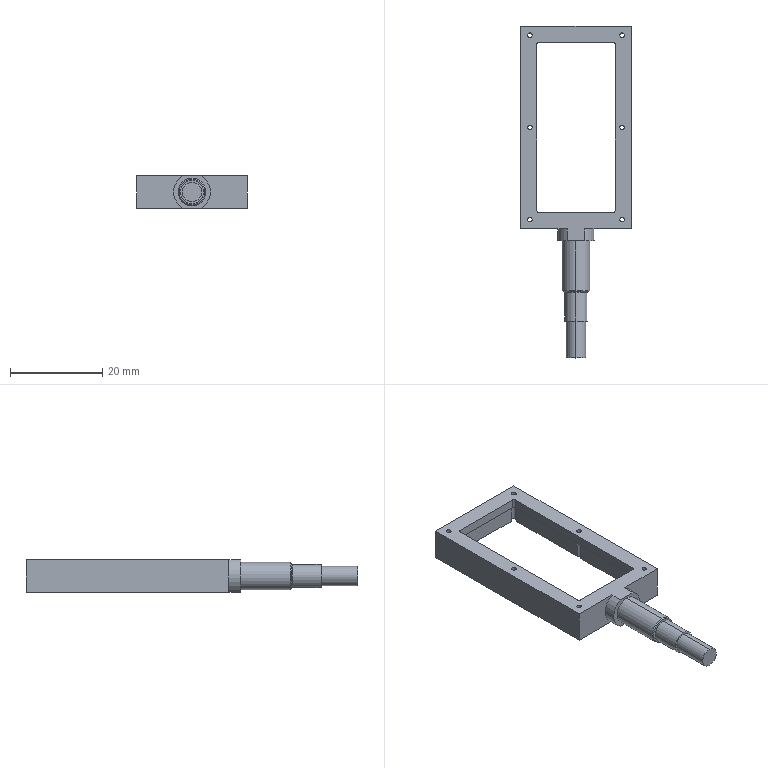NC program | NX | posted with a generic post | part box 24 x 72 x 7 mm
Lines 2081 to 3155 of 5160:
(CAVITY_MILL_COPY_COPY_COPY , TOOL : D1)
N4124 T01 M6
N4126 G54
N4128 G17 G0 G90 X-9.3 Y3.859 S9500 M3
N4130 G43 Z30. H1
N4132 Z-8.079
N4134 G94 G1 Z-9.079 F1000.
N4136 G3 X-9.5 Y3.259 R1.
N4138 G1 Y2.866 F800.
N4140 G2 X-9.634 Y2.366 R1.
N4142 X-9.134 Y2.5 R1.
N4144 G1 X-8.741
N4146 G3 X-8.141 Y2.7 R1.
N4148 G1 Z-8.079
N4150 G0 Z30.
N4152 X-9.3 Y3.859
N4154 Z-8.159
N4156 G1 Z-9.159 F1000.
N4158 G3 X-9.5 Y3.259 R1.
N4160 G1 Y2.866 F800.
N4162 G2 X-9.634 Y2.366 R1.
N4164 X-9.134 Y2.5 R1.
N4166 G1 X-8.741
N4168 G3 X-8.141 Y2.7 R1.
N4170 G1 Z-8.159
N4172 G0 Z30.
N4174 X-9.3 Y3.859
N4176 Z-8.238
N4178 G1 Z-9.238 F1000.
N4180 G3 X-9.5 Y3.259 R1.
N4182 G1 Y2.866 F800.
N4184 G2 X-9.634 Y2.366 R1.
N4186 X-9.134 Y2.5 R1.
N4188 G1 X-8.741
N4190 G3 X-8.141 Y2.7 R1.
N4192 G1 Z-8.238
N4194 G0 Z30.
N4196 X-9.3 Y3.859
N4198 Z-8.317
N4200 G1 Z-9.317 F1000.
N4202 G3 X-9.5 Y3.259 R1.
N4204 G1 Y2.866 F800.
N4206 G2 X-9.634 Y2.366 R1.
N4208 X-9.134 Y2.5 R1.
N4210 G1 X-8.741
N4212 G3 X-8.141 Y2.7 R1.
N4214 G1 Z-8.317
N4216 G0 Z30.
N4218 X-9.3 Y3.859
N4220 Z-8.397
N4222 G1 Z-9.397 F1000.
N4224 G3 X-9.5 Y3.259 R1.
N4226 G1 Y2.866 F800.
N4228 G2 X-9.634 Y2.366 R1.
N4230 X-9.134 Y2.5 R1.
N4232 G1 X-8.741
N4234 G3 X-8.141 Y2.7 R1.
N4236 G1 Z-8.397
N4238 G0 Z30.
N4240 X-9.3 Y3.859
N4242 Z-8.476
N4244 G1 Z-9.476 F1000.
N4246 G3 X-9.5 Y3.259 R1.
N4248 G1 Y2.866 F800.
N4250 G2 X-9.634 Y2.366 R1.
N4252 X-9.134 Y2.5 R1.
N4254 G1 X-8.741
N4256 G3 X-8.141 Y2.7 R1.
N4258 G1 Z-8.476
N4260 G0 Z30.
N4262 X-9.3 Y3.859
N4264 Z-8.556
N4266 G1 Z-9.556 F1000.
N4268 G3 X-9.5 Y3.259 R1.
N4270 G1 Y2.866 F800.
N4272 G2 X-9.634 Y2.366 R1.
N4274 X-9.134 Y2.5 R1.
N4276 G1 X-8.741
N4278 G3 X-8.141 Y2.7 R1.
N4280 G1 Z-8.556
N4282 G0 Z30.
N4284 X-9.3 Y3.859
N4286 Z-8.635
N4288 G1 Z-9.635 F1000.
N4290 G3 X-9.5 Y3.259 R1.
N4292 G1 Y2.866 F800.
N4294 G2 X-9.634 Y2.366 R1.
N4296 X-9.134 Y2.5 R1.
N4298 G1 X-8.741
N4300 G3 X-8.141 Y2.7 R1.
N4302 G1 Z-8.635
N4304 G0 Z30.
N4306 X-9.3 Y3.859
N4308 Z-8.714
N4310 G1 Z-9.714 F1000.
N4312 G3 X-9.5 Y3.259 R1.
N4314 G1 Y2.866 F800.
N4316 G2 X-9.634 Y2.366 R1.
N4318 X-9.134 Y2.5 R1.
N4320 G1 X-8.741
N4322 G3 X-8.141 Y2.7 R1.
N4324 G1 Z-8.714
N4326 G0 Z30.
N4328 X-9.3 Y3.859
N4330 Z-8.794
N4332 G1 Z-9.794 F1000.
N4334 G3 X-9.5 Y3.259 R1.
N4336 G1 Y2.866 F800.
N4338 G2 X-9.634 Y2.366 R1.
N4340 X-9.134 Y2.5 R1.
N4342 G1 X-8.741
N4344 G3 X-8.141 Y2.7 R1.
N4346 G1 Z-8.794
N4348 G0 Z30.
N4350 X-9.3 Y3.859
N4352 Z-8.873
N4354 G1 Z-9.873 F1000.
N4356 G3 X-9.5 Y3.259 R1.
N4358 G1 Y2.866 F800.
N4360 G2 X-9.634 Y2.366 R1.
N4362 X-9.134 Y2.5 R1.
N4364 G1 X-8.741
N4366 G3 X-8.141 Y2.7 R1.
N4368 G1 Z-8.873
N4370 G0 Z30.
N4372 X-9.3 Y3.859
N4374 Z-8.952
N4376 G1 Z-9.952 F1000.
N4378 G3 X-9.5 Y3.259 R1.
N4380 G1 Y2.866 F800.
N4382 G2 X-9.634 Y2.366 R1.
N4384 X-9.134 Y2.5 R1.
N4386 G1 X-8.741
N4388 G3 X-8.141 Y2.7 R1.
N4390 G1 Z-8.952
N4392 G0 X-9.3 Y3.859 Z-9.032
N4394 G1 Z-10.032 F1000.
N4396 G3 X-9.5 Y3.259 R1.
N4398 G1 Y2.866 F800.
N4400 G2 X-9.634 Y2.366 R1.
N4402 X-9.134 Y2.5 R1.
N4404 G1 X-8.741
N4406 G3 X-8.141 Y2.7 R1.
N4408 G1 Z-9.032
N4410 G0 X-9.3 Y3.859 Z-9.111
N4412 G1 Z-10.111 F1000.
N4414 G3 X-9.5 Y3.259 R1.
N4416 G1 Y2.866 F800.
N4418 G2 X-9.634 Y2.366 R1.
N4420 X-9.134 Y2.5 R1.
N4422 G1 X-8.741
N4424 G3 X-8.141 Y2.7 R1.
N4426 G1 Z-9.111
N4428 G0 X-9.3 Y3.859 Z-9.19
N4430 G1 Z-10.19 F1000.
N4432 G3 X-9.5 Y3.259 R1.
N4434 G1 Y2.866 F800.
N4436 G2 X-9.634 Y2.366 R1.
N4438 X-9.134 Y2.5 R1.
N4440 G1 X-8.741
N4442 G3 X-8.141 Y2.7 R1.
N4444 G1 Z-9.19
N4446 G0 X-9.3 Y3.859 Z-9.27
N4448 G1 Z-10.27 F1000.
N4450 G3 X-9.5 Y3.259 R1.
N4452 G1 Y2.866 F800.
N4454 G2 X-9.634 Y2.366 R1.
N4456 X-9.134 Y2.5 R1.
N4458 G1 X-8.741
N4460 G3 X-8.141 Y2.7 R1.
N4462 G1 Z-9.27
N4464 G0 X-9.3 Y3.859 Z-9.349
N4466 G1 Z-10.349 F1000.
N4468 G3 X-9.5 Y3.259 R1.
N4470 G1 Y2.866 F800.
N4472 G2 X-9.634 Y2.366 R1.
N4474 X-9.134 Y2.5 R1.
N4476 G1 X-8.741
N4478 G3 X-8.141 Y2.7 R1.
N4480 G1 Z-9.349
N4482 G0 X-9.3 Y3.859 Z-9.429
N4484 G1 Z-10.429 F1000.
N4486 G3 X-9.5 Y3.259 R1.
N4488 G1 Y2.866 F800.
N4490 G2 X-9.634 Y2.366 R1.
N4492 X-9.134 Y2.5 R1.
N4494 G1 X-8.741
N4496 G3 X-8.141 Y2.7 R1.
N4498 G1 Z-9.429
N4500 G0 X-9.3 Y3.859 Z-9.508
N4502 G1 Z-10.508 F1000.
N4504 G3 X-9.5 Y3.259 R1.
N4506 G1 Y2.866 F800.
N4508 G2 X-9.634 Y2.366 R1.
N4510 X-9.134 Y2.5 R1.
N4512 G1 X-8.741
N4514 G3 X-8.141 Y2.7 R1.
N4516 G1 Z-9.508
N4518 G0 X-9.3 Y3.859 Z-9.587
N4520 G1 Z-10.587 F1000.
N4522 G3 X-9.5 Y3.259 R1.
N4524 G1 Y2.866 F800.
N4526 G2 X-9.634 Y2.366 R1.
N4528 X-9.134 Y2.5 R1.
N4530 G1 X-8.741
N4532 G3 X-8.141 Y2.7 R1.
N4534 G1 Z-9.587
N4536 G0 X-9.3 Y3.859 Z-9.667
N4538 G1 Z-10.667 F1000.
N4540 G3 X-9.5 Y3.259 R1.
N4542 G1 Y2.866 F800.
N4544 G2 X-9.634 Y2.366 R1.
N4546 X-9.134 Y2.5 R1.
N4548 G1 X-8.741
N4550 G3 X-8.141 Y2.7 R1.
N4552 G1 Z-9.667
N4554 G0 X-9.3 Y3.859 Z-9.746
N4556 G1 Z-10.746 F1000.
N4558 G3 X-9.5 Y3.259 R1.
N4560 G1 Y2.866 F800.
N4562 G2 X-9.634 Y2.366 R1.
N4564 X-9.134 Y2.5 R1.
N4566 G1 X-8.741
N4568 G3 X-8.141 Y2.7 R1.
N4570 G1 Z-9.746
N4572 G0 X-9.3 Y3.859 Z-9.825
N4574 G1 Z-10.825 F1000.
N4576 G3 X-9.5 Y3.259 R1.
N4578 G1 Y2.866 F800.
N4580 G2 X-9.634 Y2.366 R1.
N4582 X-9.134 Y2.5 R1.
N4584 G1 X-8.741
N4586 G3 X-8.141 Y2.7 R1.
N4588 G1 Z-9.825
N4590 G0 X-9.3 Y3.859 Z-9.905
N4592 G1 Z-10.905 F1000.
N4594 G3 X-9.5 Y3.259 R1.
N4596 G1 Y2.866 F800.
N4598 G2 X-9.634 Y2.366 R1.
N4600 X-9.134 Y2.5 R1.
N4602 G1 X-8.741
N4604 G3 X-8.141 Y2.7 R1.
N4606 G1 Z-9.905
N4608 G0 X-9.3 Y3.859 Z-9.984
N4610 G1 Z-10.984 F1000.
N4612 G3 X-9.5 Y3.259 R1.
N4614 G1 Y2.866 F800.
N4616 G2 X-9.634 Y2.366 R1.
N4618 X-9.134 Y2.5 R1.
N4620 G1 X-8.741
N4622 G3 X-8.141 Y2.7 R1.
N4624 G1 Z-9.984
N4626 G0 X-9.3 Y3.859 Z-10.063
N4628 G1 Z-11.063 F1000.
N4630 G3 X-9.5 Y3.259 R1.
N4632 G1 Y2.866 F800.
N4634 G2 X-9.634 Y2.366 R1.
N4636 X-9.134 Y2.5 R1.
N4638 G1 X-8.741
N4640 G3 X-8.141 Y2.7 R1.
N4642 G1 Z-10.063
N4644 G0 X-9.3 Y3.859 Z-10.143
N4646 G1 Z-11.143 F1000.
N4648 G3 X-9.5 Y3.259 R1.
N4650 G1 Y2.866 F800.
N4652 G2 X-9.634 Y2.366 R1.
N4654 X-9.134 Y2.5 R1.
N4656 G1 X-8.741
N4658 G3 X-8.141 Y2.7 R1.
N4660 G1 Z-10.143
N4662 G0 X-9.3 Y3.859 Z-10.222
N4664 G1 Z-11.222 F1000.
N4666 G3 X-9.5 Y3.259 R1.
N4668 G1 Y2.866 F800.
N4670 G2 X-9.634 Y2.366 R1.
N4672 X-9.134 Y2.5 R1.
N4674 G1 X-8.741
N4676 G3 X-8.141 Y2.7 R1.
N4678 G1 Z-10.222
N4680 G0 X-9.3 Y3.859 Z-10.302
N4682 G1 Z-11.302 F1000.
N4684 G3 X-9.5 Y3.259 R1.
N4686 G1 Y2.866 F800.
N4688 G2 X-9.634 Y2.366 R1.
N4690 X-9.134 Y2.5 R1.
N4692 G1 X-8.741
N4694 G3 X-8.141 Y2.7 R1.
N4696 G1 Z-10.302
N4698 G0 X-9.3 Y3.859 Z-10.381
N4700 G1 Z-11.381 F1000.
N4702 G3 X-9.5 Y3.259 R1.
N4704 G1 Y2.866 F800.
N4706 G2 X-9.634 Y2.366 R1.
N4708 X-9.134 Y2.5 R1.
N4710 G1 X-8.741
N4712 G3 X-8.141 Y2.7 R1.
N4714 G1 Z-10.381
N4716 G0 X-9.3 Y3.859 Z-10.46
N4718 G1 Z-11.46 F1000.
N4720 G3 X-9.5 Y3.259 R1.
N4722 G1 Y2.866 F800.
N4724 G2 X-9.634 Y2.366 R1.
N4726 X-9.134 Y2.5 R1.
N4728 G1 X-8.741
N4730 G3 X-8.141 Y2.7 R1.
N4732 G1 Z-10.46
N4734 G0 X-9.3 Y3.859 Z-10.54
N4736 G1 Z-11.54 F1000.
N4738 G3 X-9.5 Y3.259 R1.
N4740 G1 Y2.866 F800.
N4742 G2 X-9.634 Y2.366 R1.
N4744 X-9.134 Y2.5 R1.
N4746 G1 X-8.741
N4748 G3 X-8.141 Y2.7 R1.
N4750 G1 Z-10.54
N4752 G0 X-9.3 Y3.859 Z-10.619
N4754 G1 Z-11.619 F1000.
N4756 G3 X-9.5 Y3.259 R1.
N4758 G1 Y2.866 F800.
N4760 G2 X-9.634 Y2.366 R1.
N4762 X-9.134 Y2.5 R1.
N4764 G1 X-8.741
N4766 G3 X-8.141 Y2.7 R1.
N4768 G1 Z-10.619
N4770 G0 X-9.3 Y3.859 Z-10.698
N4772 G1 Z-11.698 F1000.
N4774 G3 X-9.5 Y3.259 R1.
N4776 G1 Y2.866 F800.
N4778 G2 X-9.634 Y2.366 R1.
N4780 X-9.134 Y2.5 R1.
N4782 G1 X-8.741
N4784 G3 X-8.141 Y2.7 R1.
N4786 G1 Z-10.698
N4788 G0 X-9.3 Y3.859 Z-10.778
N4790 G1 Z-11.778 F1000.
N4792 G3 X-9.5 Y3.259 R1.
N4794 G1 Y2.866 F800.
N4796 G2 X-9.634 Y2.366 R1.
N4798 X-9.134 Y2.5 R1.
N4800 G1 X-8.741
N4802 G3 X-8.141 Y2.7 R1.
N4804 G1 Z-10.778
N4806 G0 X-9.3 Y3.859 Z-10.857
N4808 G1 Z-11.857 F1000.
N4810 G3 X-9.5 Y3.259 R1.
N4812 G1 Y2.866 F800.
N4814 G2 X-9.634 Y2.366 R1.
N4816 X-9.134 Y2.5 R1.
N4818 G1 X-8.741
N4820 G3 X-8.141 Y2.7 R1.
N4822 G1 Z-10.857
N4824 G0 X-9.3 Y3.859 Z-10.937
N4826 G1 Z-11.937 F1000.
N4828 G3 X-9.5 Y3.259 R1.
N4830 G1 Y2.866 F800.
N4832 G2 X-9.634 Y2.366 R1.
N4834 X-9.134 Y2.5 R1.
N4836 G1 X-8.741
N4838 G3 X-8.141 Y2.7 R1.
N4840 G1 Z-10.937
N4842 G0 X-9.3 Y3.859 Z-11.016
N4844 G1 Z-12.016 F1000.
N4846 G3 X-9.5 Y3.259 R1.
N4848 G1 Y2.866 F800.
N4850 G2 X-9.634 Y2.366 R1.
N4852 X-9.134 Y2.5 R1.
N4854 G1 X-8.741
N4856 G3 X-8.141 Y2.7 R1.
N4858 G1 Z-11.016
N4860 G0 X-9.3 Y3.859 Z-11.095
N4862 G1 Z-12.095 F1000.
N4864 G3 X-9.5 Y3.259 R1.
N4866 G1 Y2.866 F800.
N4868 G2 X-9.634 Y2.366 R1.
N4870 X-9.134 Y2.5 R1.
N4872 G1 X-8.741
N4874 G3 X-8.141 Y2.7 R1.
N4876 G1 Z-11.095
N4878 G0 X-9.3 Y3.859 Z-11.175
N4880 G1 Z-12.175 F1000.
N4882 G3 X-9.5 Y3.259 R1.
N4884 G1 Y2.866 F800.
N4886 G2 X-9.634 Y2.366 R1.
N4888 X-9.134 Y2.5 R1.
N4890 G1 X-8.741
N4892 G3 X-8.141 Y2.7 R1.
N4894 G1 Z-11.175
N4896 G0 X-9.3 Y3.859 Z-11.254
N4898 G1 Z-12.254 F1000.
N4900 G3 X-9.5 Y3.259 R1.
N4902 G1 Y2.866 F800.
N4904 G2 X-9.634 Y2.366 R1.
N4906 X-9.134 Y2.5 R1.
N4908 G1 X-8.741
N4910 G3 X-8.141 Y2.7 R1.
N4912 G1 Z-11.254
N4914 G0 X-9.3 Y3.859 Z-11.333
N4916 G1 Z-12.333 F1000.
N4918 G3 X-9.5 Y3.259 R1.
N4920 G1 Y2.866 F800.
N4922 G2 X-9.634 Y2.366 R1.
N4924 X-9.134 Y2.5 R1.
N4926 G1 X-8.741
N4928 G3 X-8.141 Y2.7 R1.
N4930 G1 Z-11.333
N4932 G0 X-9.3 Y3.859 Z-11.413
N4934 G1 Z-12.413 F1000.
N4936 G3 X-9.5 Y3.259 R1.
N4938 G1 Y2.866 F800.
N4940 G2 X-9.634 Y2.366 R1.
N4942 X-9.134 Y2.5 R1.
N4944 G1 X-8.741
N4946 G3 X-8.141 Y2.7 R1.
N4948 G1 Z-11.413
N4950 G0 X-9.3 Y3.859 Z-11.492
N4952 G1 Z-12.492 F1000.
N4954 G3 X-9.5 Y3.259 R1.
N4956 G1 Y2.866 F800.
N4958 G2 X-9.634 Y2.366 R1.
N4960 X-9.134 Y2.5 R1.
N4962 G1 X-8.741
N4964 G3 X-8.141 Y2.7 R1.
N4966 G1 Z-11.492
N4968 G0 X-9.3 Y3.859 Z-11.571
N4970 G1 Z-12.571 F1000.
N4972 G3 X-9.5 Y3.259 R1.
N4974 G1 Y2.866 F800.
N4976 G2 X-9.634 Y2.366 R1.
N4978 X-9.134 Y2.5 R1.
N4980 G1 X-8.741
N4982 G3 X-8.141 Y2.7 R1.
N4984 G1 Z-11.571
N4986 G0 X-9.3 Y3.859 Z-11.651
N4988 G1 Z-12.651 F1000.
N4990 G3 X-9.5 Y3.259 R1.
N4992 G1 Y2.866 F800.
N4994 G2 X-9.634 Y2.366 R1.
N4996 X-9.134 Y2.5 R1.
N4998 G1 X-8.741
N5000 G3 X-8.141 Y2.7 R1.
N5002 G1 Z-11.651
N5004 G0 X-9.3 Y3.859 Z-11.73
N5006 G1 Z-12.73 F1000.
N5008 G3 X-9.5 Y3.259 R1.
N5010 G1 Y2.866 F800.
N5012 G2 X-9.634 Y2.366 R1.
N5014 X-9.134 Y2.5 R1.
N5016 G1 X-8.741
N5018 G3 X-8.141 Y2.7 R1.
N5020 G1 Z-11.73
N5022 G0 X-9.3 Y3.859 Z-11.81
N5024 G1 Z-12.81 F1000.
N5026 G3 X-9.5 Y3.259 R1.
N5028 G1 Y2.866 F800.
N5030 G2 X-9.634 Y2.366 R1.
N5032 X-9.134 Y2.5 R1.
N5034 G1 X-8.741
N5036 G3 X-8.141 Y2.7 R1.
N5038 G1 Z-11.81
N5040 G0 X-9.3 Y3.859 Z-11.889
N5042 G1 Z-12.889 F1000.
N5044 G3 X-9.5 Y3.259 R1.
N5046 G1 Y2.866 F800.
N5048 G2 X-9.634 Y2.366 R1.
N5050 X-9.134 Y2.5 R1.
N5052 G1 X-8.741
N5054 G3 X-8.141 Y2.7 R1.
N5056 G1 Z-11.889
N5058 G0 X-9.3 Y3.859 Z-11.968
N5060 G1 Z-12.968 F1000.
N5062 G3 X-9.5 Y3.259 R1.
N5064 G1 Y2.866 F800.
N5066 G2 X-9.634 Y2.366 R1.
N5068 X-9.134 Y2.5 R1.
N5070 G1 X-8.741
N5072 G3 X-8.141 Y2.7 R1.
N5074 G1 Z-11.968
N5076 G0 X-9.3 Y3.859 Z-12.048
N5078 G1 Z-13.048 F1000.
N5080 G3 X-9.5 Y3.259 R1.
N5082 G1 Y2.866 F800.
N5084 G2 X-9.634 Y2.366 R1.
N5086 X-9.134 Y2.5 R1.
N5088 G1 X-8.741
N5090 G3 X-8.141 Y2.7 R1.
N5092 G1 Z-12.048
N5094 G0 X-9.3 Y3.859 Z-12.127
N5096 G1 Z-13.127 F1000.
N5098 G3 X-9.5 Y3.259 R1.
N5100 G1 Y2.866 F800.
N5102 G2 X-9.634 Y2.366 R1.
N5104 X-9.134 Y2.5 R1.
N5106 G1 X-8.741
N5108 G3 X-8.141 Y2.7 R1.
N5110 G1 Z-12.127
N5112 G0 X-9.3 Y3.859 Z-12.206
N5114 G1 Z-13.206 F1000.
N5116 G3 X-9.5 Y3.259 R1.
N5118 G1 Y2.866 F800.
N5120 G2 X-9.634 Y2.366 R1.
N5122 X-9.134 Y2.5 R1.
N5124 G1 X-8.741
N5126 G3 X-8.141 Y2.7 R1.
N5128 G1 Z-12.206
N5130 G0 X-9.3 Y3.859 Z-12.286
N5132 G1 Z-13.286 F1000.
N5134 G3 X-9.5 Y3.259 R1.
N5136 G1 Y2.866 F800.
N5138 G2 X-9.634 Y2.366 R1.
N5140 X-9.134 Y2.5 R1.
N5142 G1 X-8.741
N5144 G3 X-8.141 Y2.7 R1.
N5146 G1 Z-12.286
N5148 G0 X-9.3 Y3.859 Z-12.365
N5150 G1 Z-13.365 F1000.
N5152 G3 X-9.5 Y3.259 R1.
N5154 G1 Y2.866 F800.
N5156 G2 X-9.634 Y2.366 R1.
N5158 X-9.134 Y2.5 R1.
N5160 G1 X-8.741
N5162 G3 X-8.141 Y2.7 R1.
N5164 G1 Z-12.365
N5166 G0 X-9.3 Y3.859 Z-12.444
N5168 G1 Z-13.444 F1000.
N5170 G3 X-9.5 Y3.259 R1.
N5172 G1 Y2.866 F800.
N5174 G2 X-9.634 Y2.366 R1.
N5176 X-9.134 Y2.5 R1.
N5178 G1 X-8.741
N5180 G3 X-8.141 Y2.7 R1.
N5182 G1 Z-12.444
N5184 G0 X-9.3 Y3.859 Z-12.524
N5186 G1 Z-13.524 F1000.
N5188 G3 X-9.5 Y3.259 R1.
N5190 G1 Y2.866 F800.
N5192 G2 X-9.634 Y2.366 R1.
N5194 X-9.134 Y2.5 R1.
N5196 G1 X-8.741
N5198 G3 X-8.141 Y2.7 R1.
N5200 G1 Z-12.524
N5202 G0 X-9.3 Y3.859 Z-12.603
N5204 G1 Z-13.603 F1000.
N5206 G3 X-9.5 Y3.259 R1.
N5208 G1 Y2.866 F800.
N5210 G2 X-9.634 Y2.366 R1.
N5212 X-9.134 Y2.5 R1.
N5214 G1 X-8.741
N5216 G3 X-8.141 Y2.7 R1.
N5218 G1 Z-12.603
N5220 G0 X-9.3 Y3.859 Z-12.683
N5222 G1 Z-13.683 F1000.
N5224 G3 X-9.5 Y3.259 R1.
N5226 G1 Y2.866 F800.
N5228 G2 X-9.634 Y2.366 R1.
N5230 X-9.134 Y2.5 R1.
N5232 G1 X-8.741
N5234 G3 X-8.141 Y2.7 R1.
N5236 G1 Z-12.683
N5238 G0 X-9.3 Y3.859 Z-12.762
N5240 G1 Z-13.762 F1000.
N5242 G3 X-9.5 Y3.259 R1.
N5244 G1 Y2.866 F800.
N5246 G2 X-9.634 Y2.366 R1.
N5248 X-9.134 Y2.5 R1.
N5250 G1 X-8.741
N5252 G3 X-8.141 Y2.7 R1.
N5254 G1 Z-12.762
N5256 G0 X-9.3 Y3.859 Z-12.841
N5258 G1 Z-13.841 F1000.
N5260 G3 X-9.5 Y3.259 R1.
N5262 G1 Y2.866 F800.
N5264 G2 X-9.634 Y2.366 R1.
N5266 X-9.134 Y2.5 R1.
N5268 G1 X-8.741
N5270 G3 X-8.141 Y2.7 R1.
N5272 G1 Z-12.841
N5274 G0 X-9.3 Y3.859 Z-12.921
N5276 G1 Z-13.921 F1000.
N5278 G3 X-9.5 Y3.259 R1.
N5280 G1 Y2.866 F800.
N5282 G2 X-9.634 Y2.366 R1.
N5284 X-9.134 Y2.5 R1.
N5286 G1 X-8.741
N5288 G3 X-8.141 Y2.7 R1.
N5290 G1 Z-12.921
N5292 G0 X-9.3 Y3.859 Z-13.
N5294 G1 Z-14. F1000.
N5296 G3 X-9.5 Y3.259 R1.
N5298 G1 Y2.866 F800.
N5300 G2 X-9.634 Y2.366 R1.
N5302 X-9.134 Y2.5 R1.
N5304 G1 X-8.741
N5306 G3 X-8.141 Y2.7 R1.
N5308 G1 Z-13.
N5310 G0 Z30.
N5312 X-7.8 Y5.348
N5314 Z-13.08
N5316 G1 Z-14.08 F1000.
N5318 G3 X-8. Y4.748 R1.
N5320 G1 Y4. F800.
N5322 X-7.252
N5324 G3 X-6.652 Y4.2 R1.
N5326 G1 Z-13.08
N5328 G0 X-7.8 Y5.348 Z-13.16
N5330 G1 Z-14.16 F1000.
N5332 G3 X-8. Y4.748 R1.
N5334 G1 Y4. F800.
N5336 X-7.252
N5338 G3 X-6.652 Y4.2 R1.
N5340 G1 Z-13.16
N5342 G0 X-7.8 Y5.348 Z-13.24
N5344 G1 Z-14.24 F1000.
N5346 G3 X-8. Y4.748 R1.
N5348 G1 Y4. F800.
N5350 X-7.252
N5352 G3 X-6.652 Y4.2 R1.
N5354 G1 Z-13.24
N5356 G0 X-7.8 Y5.348 Z-13.32
N5358 G1 Z-14.32 F1000.
N5360 G3 X-8. Y4.748 R1.
N5362 G1 Y4. F800.
N5364 X-7.252
N5366 G3 X-6.652 Y4.2 R1.
N5368 G1 Z-13.32
N5370 G0 X-7.8 Y5.348 Z-13.4
N5372 G1 Z-14.4 F1000.
N5374 G3 X-8. Y4.748 R1.
N5376 G1 Y4. F800.
N5378 X-7.252
N5380 G3 X-6.652 Y4.2 R1.
N5382 G1 Z-13.4
N5384 G0 X-7.8 Y5.348 Z-13.48
N5386 G1 Z-14.48 F1000.
N5388 G3 X-8. Y4.748 R1.
N5390 G1 Y4. F800.
N5392 X-7.252
N5394 G3 X-6.652 Y4.2 R1.
N5396 G1 Z-13.48
N5398 G0 X-7.8 Y5.348 Z-13.56
N5400 G1 Z-14.56 F1000.
N5402 G3 X-8. Y4.748 R1.
N5404 G1 Y4. F800.
N5406 X-7.252
N5408 G3 X-6.652 Y4.2 R1.
N5410 G1 Z-13.56
N5412 G0 X-7.8 Y5.348 Z-13.64
N5414 G1 Z-14.64 F1000.
N5416 G3 X-8. Y4.748 R1.
N5418 G1 Y4. F800.
N5420 X-7.252
N5422 G3 X-6.652 Y4.2 R1.
N5424 G1 Z-13.64
N5426 G0 X-7.8 Y5.348 Z-13.72
N5428 G1 Z-14.72 F1000.
N5430 G3 X-8. Y4.748 R1.
N5432 G1 Y4. F800.
N5434 X-7.252
N5436 G3 X-6.652 Y4.2 R1.
N5438 G1 Z-13.72
N5440 G0 X-7.8 Y5.348 Z-13.8
N5442 G1 Z-14.8 F1000.
N5444 G3 X-8. Y4.748 R1.
N5446 G1 Y4. F800.
N5448 X-7.252
N5450 G3 X-6.652 Y4.2 R1.
N5452 G1 Z-13.8
N5454 G0 X-7.8 Y5.348 Z-13.88
N5456 G1 Z-14.88 F1000.
N5458 G3 X-8. Y4.748 R1.
N5460 G1 Y4. F800.
N5462 X-7.252
N5464 G3 X-6.652 Y4.2 R1.
N5466 G1 Z-13.88
N5468 G0 X-7.8 Y5.348 Z-13.96
N5470 G1 Z-14.96 F1000.
N5472 G3 X-8. Y4.748 R1.
N5474 G1 Y4. F800.
N5476 X-7.252
N5478 G3 X-6.652 Y4.2 R1.
N5480 G1 Z-13.96
N5482 G0 X-7.8 Y5.348 Z-14.04
N5484 G1 Z-15.04 F1000.
N5486 G3 X-8. Y4.748 R1.
N5488 G1 Y4. F800.
N5490 X-7.252
N5492 G3 X-6.652 Y4.2 R1.
N5494 G1 Z-14.04
N5496 G0 X-7.8 Y5.348 Z-14.12
N5498 G1 Z-15.12 F1000.
N5500 G3 X-8. Y4.748 R1.
N5502 G1 Y4. F800.
N5504 X-7.252
N5506 G3 X-6.652 Y4.2 R1.
N5508 G1 Z-14.12
N5510 G0 X-7.8 Y5.348 Z-14.2
N5512 G1 Z-15.2 F1000.
N5514 G3 X-8. Y4.748 R1.
N5516 G1 Y4. F800.
N5518 X-7.252
N5520 G3 X-6.652 Y4.2 R1.
N5522 G1 Z-14.2
N5524 G0 X-7.8 Y5.348 Z-14.28
N5526 G1 Z-15.28 F1000.
N5528 G3 X-8. Y4.748 R1.
N5530 G1 Y4. F800.
N5532 X-7.252
N5534 G3 X-6.652 Y4.2 R1.
N5536 G1 Z-14.28
N5538 G0 X-7.8 Y5.348 Z-14.36
N5540 G1 Z-15.36 F1000.
N5542 G3 X-8. Y4.748 R1.
N5544 G1 Y4. F800.
N5546 X-7.252
N5548 G3 X-6.652 Y4.2 R1.
N5550 G1 Z-14.36
N5552 G0 X-7.8 Y5.348 Z-14.44
N5554 G1 Z-15.44 F1000.
N5556 G3 X-8. Y4.748 R1.
N5558 G1 Y4. F800.
N5560 X-7.252
N5562 G3 X-6.652 Y4.2 R1.
N5564 G1 Z-14.44
N5566 G0 X-7.8 Y5.348 Z-14.52
N5568 G1 Z-15.52 F1000.
N5570 G3 X-8. Y4.748 R1.
N5572 G1 Y4. F800.
N5574 X-7.252
N5576 G3 X-6.652 Y4.2 R1.
N5578 G1 Z-14.52
N5580 G0 X-7.8 Y5.348 Z-14.6
N5582 G1 Z-15.6 F1000.
N5584 G3 X-8. Y4.748 R1.
N5586 G1 Y4. F800.
N5588 X-7.252
N5590 G3 X-6.652 Y4.2 R1.
N5592 G1 Z-14.6
N5594 G0 X-7.8 Y5.348 Z-14.68
N5596 G1 Z-15.68 F1000.
N5598 G3 X-8. Y4.748 R1.
N5600 G1 Y4. F800.
N5602 X-7.252
N5604 G3 X-6.652 Y4.2 R1.
N5606 G1 Z-14.68
N5608 G0 X-7.8 Y5.348 Z-14.76
N5610 G1 Z-15.76 F1000.
N5612 G3 X-8. Y4.748 R1.
N5614 G1 Y4. F800.
N5616 X-7.252
N5618 G3 X-6.652 Y4.2 R1.
N5620 G1 Z-14.76
N5622 G0 X-7.8 Y5.348 Z-14.84
N5624 G1 Z-15.84 F1000.
N5626 G3 X-8. Y4.748 R1.
N5628 G1 Y4. F800.
N5630 X-7.252
N5632 G3 X-6.652 Y4.2 R1.
N5634 G1 Z-14.84
N5636 G0 X-7.8 Y5.348 Z-14.92
N5638 G1 Z-15.92 F1000.
N5640 G3 X-8. Y4.748 R1.
N5642 G1 Y4. F800.
N5644 X-7.252
N5646 G3 X-6.652 Y4.2 R1.
N5648 G1 Z-14.92
N5650 G0 X-7.8 Y5.348 Z-15.
N5652 G1 Z-16. F1000.
N5654 G3 X-8. Y4.748 R1.
N5656 G1 Y4. F800.
N5658 X-7.252
N5660 G3 X-6.652 Y4.2 R1.
N5662 G1 Z-15.
N5664 G0 Z30.
N5666 X6.652
N5668 Z-13.08
N5670 G1 Z-14.08 F1000.
N5672 G3 X7.252 Y4. R1.
N5674 G1 X8. F800.
N5676 Y4.748
N5678 G3 X7.8 Y5.348 R1.
N5680 G1 Z-13.08
N5682 G0 X6.652 Y4.2 Z-13.16
N5684 G1 Z-14.16 F1000.
N5686 G3 X7.252 Y4. R1.
N5688 G1 X8. F800.
N5690 Y4.748
N5692 G3 X7.8 Y5.348 R1.
N5694 G1 Z-13.16
N5696 G0 X6.652 Y4.2 Z-13.24
N5698 G1 Z-14.24 F1000.
N5700 G3 X7.252 Y4. R1.
N5702 G1 X8. F800.
N5704 Y4.748
N5706 G3 X7.8 Y5.348 R1.
N5708 G1 Z-13.24
N5710 G0 X6.652 Y4.2 Z-13.32
N5712 G1 Z-14.32 F1000.
N5714 G3 X7.252 Y4. R1.
N5716 G1 X8. F800.
N5718 Y4.748
N5720 G3 X7.8 Y5.348 R1.
N5722 G1 Z-13.32
N5724 G0 X6.652 Y4.2 Z-13.4
N5726 G1 Z-14.4 F1000.
N5728 G3 X7.252 Y4. R1.
N5730 G1 X8. F800.
N5732 Y4.748
N5734 G3 X7.8 Y5.348 R1.
N5736 G1 Z-13.4
N5738 G0 X6.652 Y4.2 Z-13.48
N5740 G1 Z-14.48 F1000.
N5742 G3 X7.252 Y4. R1.
N5744 G1 X8. F800.
N5746 Y4.748
N5748 G3 X7.8 Y5.348 R1.
N5750 G1 Z-13.48
N5752 G0 X6.652 Y4.2 Z-13.56
N5754 G1 Z-14.56 F1000.
N5756 G3 X7.252 Y4. R1.
N5758 G1 X8. F800.
N5760 Y4.748
N5762 G3 X7.8 Y5.348 R1.
N5764 G1 Z-13.56
N5766 G0 X6.652 Y4.2 Z-13.64
N5768 G1 Z-14.64 F1000.
N5770 G3 X7.252 Y4. R1.
N5772 G1 X8. F800.
N5774 Y4.748
N5776 G3 X7.8 Y5.348 R1.
N5778 G1 Z-13.64
N5780 G0 X6.652 Y4.2 Z-13.72
N5782 G1 Z-14.72 F1000.
N5784 G3 X7.252 Y4. R1.
N5786 G1 X8. F800.
N5788 Y4.748
N5790 G3 X7.8 Y5.348 R1.
N5792 G1 Z-13.72
N5794 G0 X6.652 Y4.2 Z-13.8
N5796 G1 Z-14.8 F1000.
N5798 G3 X7.252 Y4. R1.
N5800 G1 X8. F800.
N5802 Y4.748
N5804 G3 X7.8 Y5.348 R1.
N5806 G1 Z-13.8
N5808 G0 X6.652 Y4.2 Z-13.88
N5810 G1 Z-14.88 F1000.
N5812 G3 X7.252 Y4. R1.
N5814 G1 X8. F800.
N5816 Y4.748
N5818 G3 X7.8 Y5.348 R1.
N5820 G1 Z-13.88
N5822 G0 X6.652 Y4.2 Z-13.96
N5824 G1 Z-14.96 F1000.
N5826 G3 X7.252 Y4. R1.
N5828 G1 X8. F800.
N5830 Y4.748
N5832 G3 X7.8 Y5.348 R1.
N5834 G1 Z-13.96
N5836 G0 X6.652 Y4.2 Z-14.04
N5838 G1 Z-15.04 F1000.
N5840 G3 X7.252 Y4. R1.
N5842 G1 X8. F800.
N5844 Y4.748
N5846 G3 X7.8 Y5.348 R1.
N5848 G1 Z-14.04
N5850 G0 X6.652 Y4.2 Z-14.12
N5852 G1 Z-15.12 F1000.
N5854 G3 X7.252 Y4. R1.
N5856 G1 X8. F800.
N5858 Y4.748
N5860 G3 X7.8 Y5.348 R1.
N5862 G1 Z-14.12
N5864 G0 X6.652 Y4.2 Z-14.2
N5866 G1 Z-15.2 F1000.
N5868 G3 X7.252 Y4. R1.
N5870 G1 X8. F800.
N5872 Y4.748
N5874 G3 X7.8 Y5.348 R1.
N5876 G1 Z-14.2
N5878 G0 X6.652 Y4.2 Z-14.28
N5880 G1 Z-15.28 F1000.
N5882 G3 X7.252 Y4. R1.
N5884 G1 X8. F800.
N5886 Y4.748
N5888 G3 X7.8 Y5.348 R1.
N5890 G1 Z-14.28
N5892 G0 X6.652 Y4.2 Z-14.36
N5894 G1 Z-15.36 F1000.
N5896 G3 X7.252 Y4. R1.
N5898 G1 X8. F800.
N5900 Y4.748
N5902 G3 X7.8 Y5.348 R1.
N5904 G1 Z-14.36
N5906 G0 X6.652 Y4.2 Z-14.44
N5908 G1 Z-15.44 F1000.
N5910 G3 X7.252 Y4. R1.
N5912 G1 X8. F800.
N5914 Y4.748
N5916 G3 X7.8 Y5.348 R1.
N5918 G1 Z-14.44
N5920 G0 X6.652 Y4.2 Z-14.52
N5922 G1 Z-15.52 F1000.
N5924 G3 X7.252 Y4. R1.
N5926 G1 X8. F800.
N5928 Y4.748
N5930 G3 X7.8 Y5.348 R1.
N5932 G1 Z-14.52
N5934 G0 X6.652 Y4.2 Z-14.6
N5936 G1 Z-15.6 F1000.
N5938 G3 X7.252 Y4. R1.
N5940 G1 X8. F800.
N5942 Y4.748
N5944 G3 X7.8 Y5.348 R1.
N5946 G1 Z-14.6
N5948 G0 X6.652 Y4.2 Z-14.68
N5950 G1 Z-15.68 F1000.
N5952 G3 X7.252 Y4. R1.
N5954 G1 X8. F800.
N5956 Y4.748
N5958 G3 X7.8 Y5.348 R1.
N5960 G1 Z-14.68
N5962 G0 X6.652 Y4.2 Z-14.76
N5964 G1 Z-15.76 F1000.
N5966 G3 X7.252 Y4. R1.
N5968 G1 X8. F800.
N5970 Y4.748
N5972 G3 X7.8 Y5.348 R1.
N5974 G1 Z-14.76
N5976 G0 X6.652 Y4.2 Z-14.84
N5978 G1 Z-15.84 F1000.
N5980 G3 X7.252 Y4. R1.
N5982 G1 X8. F800.
N5984 Y4.748
N5986 G3 X7.8 Y5.348 R1.
N5988 G1 Z-14.84
N5990 G0 X6.652 Y4.2 Z-14.92
N5992 G1 Z-15.92 F1000.
N5994 G3 X7.252 Y4. R1.
N5996 G1 X8. F800.
N5998 Y4.748
N6000 G3 X7.8 Y5.348 R1.
N6002 G1 Z-14.92
N6004 G0 X6.652 Y4.2 Z-15.
N6006 G1 Z-16. F1000.
N6008 G3 X7.252 Y4. R1.
N6010 G1 X8. F800.
N6012 Y4.748
N6014 G3 X7.8 Y5.348 R1.
N6016 G1 Z-15.
N6018 G0 Z30.
N6020 X8.141 Y2.7
N6022 Z-8.079
N6024 G1 Z-9.079 F1000.
N6026 G3 X8.741 Y2.5 R1.
N6028 G1 X9.134 F800.
N6030 G2 X9.634 Y2.366 R1.
N6032 X9.5 Y2.866 R1.
N6034 G1 Y3.259
N6036 G3 X9.3 Y3.859 R1.
N6038 G1 Z-8.079
N6040 G0 Z30.
N6042 X8.141 Y2.7
N6044 Z-8.159
N6046 G1 Z-9.159 F1000.
N6048 G3 X8.741 Y2.5 R1.
N6050 G1 X9.134 F800.
N6052 G2 X9.634 Y2.366 R1.
N6054 X9.5 Y2.866 R1.
N6056 G1 Y3.259
N6058 G3 X9.3 Y3.859 R1.
N6060 G1 Z-8.159
N6062 G0 Z30.
N6064 X8.141 Y2.7
N6066 Z-8.238
N6068 G1 Z-9.238 F1000.
N6070 G3 X8.741 Y2.5 R1.
N6072 G1 X9.134 F800.
N6074 G2 X9.634 Y2.366 R1.
N6076 X9.5 Y2.866 R1.
N6078 G1 Y3.259
N6080 G3 X9.3 Y3.859 R1.
N6082 G1 Z-8.238
N6084 G0 Z30.
N6086 X8.141 Y2.7
N6088 Z-8.317
N6090 G1 Z-9.317 F1000.
N6092 G3 X8.741 Y2.5 R1.
N6094 G1 X9.134 F800.
N6096 G2 X9.634 Y2.366 R1.
N6098 X9.5 Y2.866 R1.
N6100 G1 Y3.259
N6102 G3 X9.3 Y3.859 R1.
N6104 G1 Z-8.317
N6106 G0 Z30.
N6108 X8.141 Y2.7
N6110 Z-8.397
N6112 G1 Z-9.397 F1000.
N6114 G3 X8.741 Y2.5 R1.
N6116 G1 X9.134 F800.
N6118 G2 X9.634 Y2.366 R1.
N6120 X9.5 Y2.866 R1.
N6122 G1 Y3.259
N6124 G3 X9.3 Y3.859 R1.
N6126 G1 Z-8.397
N6128 G0 Z30.
N6130 X8.141 Y2.7
N6132 Z-8.476
N6134 G1 Z-9.476 F1000.
N6136 G3 X8.741 Y2.5 R1.
N6138 G1 X9.134 F800.
N6140 G2 X9.634 Y2.366 R1.
N6142 X9.5 Y2.866 R1.
N6144 G1 Y3.259
N6146 G3 X9.3 Y3.859 R1.
N6148 G1 Z-8.476
N6150 G0 Z30.
N6152 X8.141 Y2.7
N6154 Z-8.556
N6156 G1 Z-9.556 F1000.
N6158 G3 X8.741 Y2.5 R1.
N6160 G1 X9.134 F800.
N6162 G2 X9.634 Y2.366 R1.
N6164 X9.5 Y2.866 R1.
N6166 G1 Y3.259
N6168 G3 X9.3 Y3.859 R1.
N6170 G1 Z-8.556
N6172 G0 Z30.
N6174 X8.141 Y2.7
N6176 Z-8.635
N6178 G1 Z-9.635 F1000.
N6180 G3 X8.741 Y2.5 R1.
N6182 G1 X9.134 F800.
N6184 G2 X9.634 Y2.366 R1.
N6186 X9.5 Y2.866 R1.
N6188 G1 Y3.259
N6190 G3 X9.3 Y3.859 R1.
N6192 G1 Z-8.635
N6194 G0 Z30.
N6196 X8.141 Y2.7
N6198 Z-8.714
N6200 G1 Z-9.714 F1000.
N6202 G3 X8.741 Y2.5 R1.
N6204 G1 X9.134 F800.
N6206 G2 X9.634 Y2.366 R1.
N6208 X9.5 Y2.866 R1.
N6210 G1 Y3.259
N6212 G3 X9.3 Y3.859 R1.
N6214 G1 Z-8.714
N6216 G0 Z30.
N6218 X8.141 Y2.7
N6220 Z-8.794
N6222 G1 Z-9.794 F1000.
N6224 G3 X8.741 Y2.5 R1.
N6226 G1 X9.134 F800.
N6228 G2 X9.634 Y2.366 R1.
N6230 X9.5 Y2.866 R1.
N6232 G1 Y3.259
N6234 G3 X9.3 Y3.859 R1.
N6236 G1 Z-8.794
N6238 G0 Z30.
N6240 X8.141 Y2.7
N6242 Z-8.873
N6244 G1 Z-9.873 F1000.
N6246 G3 X8.741 Y2.5 R1.
N6248 G1 X9.134 F800.
N6250 G2 X9.634 Y2.366 R1.
N6252 X9.5 Y2.866 R1.
N6254 G1 Y3.259
N6256 G3 X9.3 Y3.859 R1.
N6258 G1 Z-8.873
N6260 G0 Z30.
N6262 X8.141 Y2.7
N6264 Z-8.952
N6266 G1 Z-9.952 F1000.